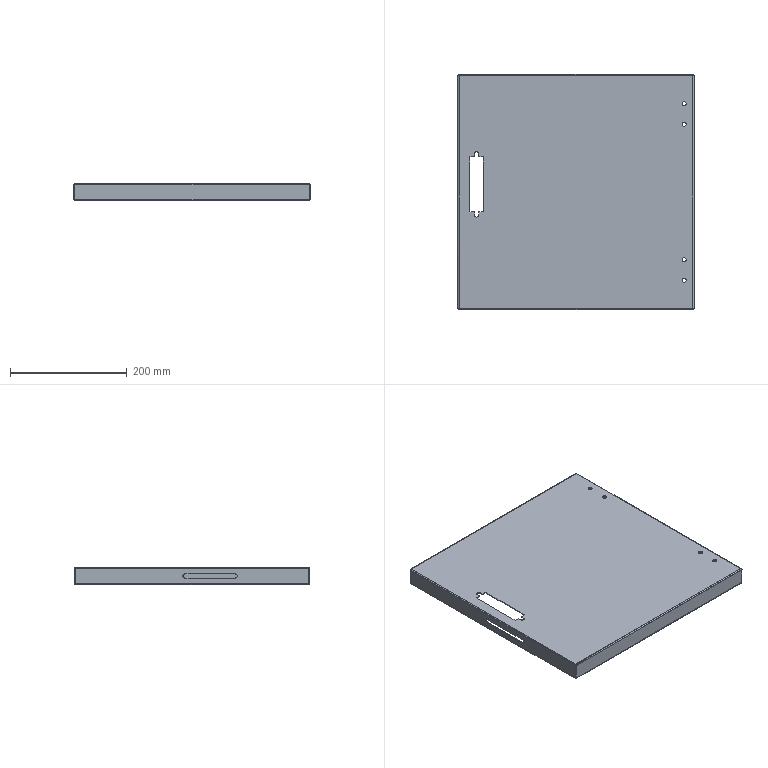Part | 1 solid | 95 faces | box 404 x 402 x 30 mm | volume 264504 mm3 | plane 50 | cylinder 29 | spline 16 | commonest cylinder face diameters 7 x13 1.473 x8 3.873 x8